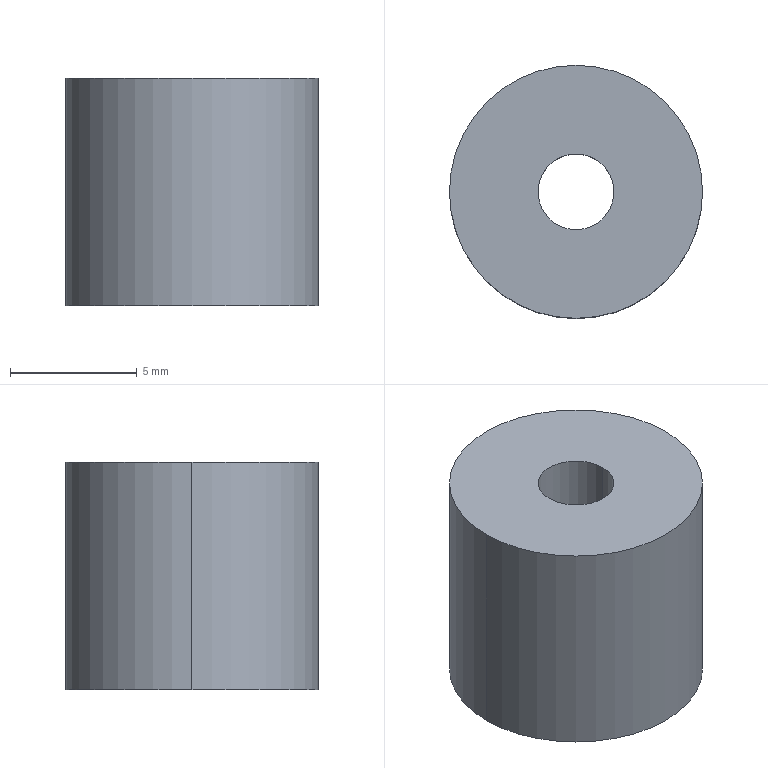Part | STEP file | 1 solid | 9 faces | box 10 x 10 x 9 mm | volume 537.212 mm3 | cylinder 6 | plane 3 | commonest cylinder face diameters 3 x2 6 x2 10 x2
STEP:
#1=CARTESIAN_POINT('',(0.,0.,0.));
#2=DIRECTION('',(0.,0.,1.));
#3=DIRECTION('',(1.,0.,0.));
#4=AXIS2_PLACEMENT_3D('',#1,#2,#3);
#5=CARTESIAN_POINT('',(1.5,0.,-4.));
#6=VERTEX_POINT('',#5);
#7=CARTESIAN_POINT('',(1.5,0.,0.));
#8=VERTEX_POINT('',#7);
#9=CARTESIAN_POINT('',(1.5,0.,0.));
#10=DIRECTION('',(0.,0.,1.));
#11=VECTOR('',#10,1.);
#12=LINE('',#9,#11);
#13=CARTESIAN_POINT('',(0.,0.,0.));
#14=DIRECTION('',(0.,0.,1.));
#15=DIRECTION('',(1.,0.,0.));
#16=AXIS2_PLACEMENT_3D('',#13,#14,#15);
#17=CYLINDRICAL_SURFACE('',#16,1.5);
#18=CARTESIAN_POINT('',(6.283,0.));
#19=DIRECTION('',(0.,1.));
#20=VECTOR('',#19,1.);
#21=LINE('',#18,#20);
#22=(GEOMETRIC_REPRESENTATION_CONTEXT(2)PARAMETRIC_REPRESENTATION_CONTEXT()REPRESENTATION_CONTEXT('',''));
#23=DEFINITIONAL_REPRESENTATION('',(#21),#22);
#24=PCURVE('',#17,#23);
#25=CARTESIAN_POINT('',(0.,0.,0.));
#26=DIRECTION('',(0.,0.,1.));
#27=DIRECTION('',(1.,0.,0.));
#28=AXIS2_PLACEMENT_3D('',#25,#26,#27);
#29=CYLINDRICAL_SURFACE('',#28,1.5);
#30=CARTESIAN_POINT('',(0.,0.));
#31=DIRECTION('',(0.,1.));
#32=VECTOR('',#31,1.);
#33=LINE('',#30,#32);
#34=(GEOMETRIC_REPRESENTATION_CONTEXT(2)PARAMETRIC_REPRESENTATION_CONTEXT()REPRESENTATION_CONTEXT('',''));
#35=DEFINITIONAL_REPRESENTATION('',(#33),#34);
#36=PCURVE('',#29,#35);
#37=SURFACE_CURVE('',#12,(#24,#36),.PCURVE_S1.);
#38=EDGE_CURVE('',#6,#8,#37,.T.);
#39=ORIENTED_EDGE('',*,*,#38,.T.);
#40=CARTESIAN_POINT('',(-1.5,0.,0.));
#41=VERTEX_POINT('',#40);
#42=CARTESIAN_POINT('',(0.,0.,0.));
#43=DIRECTION('',(0.,0.,1.));
#44=DIRECTION('',(1.,0.,0.));
#45=AXIS2_PLACEMENT_3D('',#42,#43,#44);
#46=CIRCLE('',#45,1.5);
#47=CARTESIAN_POINT('',(0.,0.));
#48=DIRECTION('',(1.,0.));
#49=VECTOR('',#48,1.);
#50=LINE('',#47,#49);
#51=(GEOMETRIC_REPRESENTATION_CONTEXT(2)PARAMETRIC_REPRESENTATION_CONTEXT()REPRESENTATION_CONTEXT('',''));
#52=DEFINITIONAL_REPRESENTATION('',(#50),#51);
#53=PCURVE('',#17,#52);
#54=CARTESIAN_POINT('',(1.5,0.,0.));
#55=DIRECTION('',(0.,0.,1.));
#56=DIRECTION('',(1.,0.,0.));
#57=AXIS2_PLACEMENT_3D('',#54,#55,#56);
#58=PLANE('',#57);
#59=CARTESIAN_POINT('',(-1.5,0.));
#60=DIRECTION('',(1.,0.));
#61=AXIS2_PLACEMENT_2D('',#59,#60);
#62=CIRCLE('',#61,1.5);
#63=(GEOMETRIC_REPRESENTATION_CONTEXT(2)PARAMETRIC_REPRESENTATION_CONTEXT()REPRESENTATION_CONTEXT('',''));
#64=DEFINITIONAL_REPRESENTATION('',(#62),#63);
#65=PCURVE('',#58,#64);
#66=SURFACE_CURVE('',#46,(#53,#65),.PCURVE_S1.);
#67=EDGE_CURVE('',#41,#8,#66,.T.);
#68=ORIENTED_EDGE('',*,*,#67,.F.);
#69=CARTESIAN_POINT('',(-1.5,0.,-4.));
#70=VERTEX_POINT('',#69);
#71=CARTESIAN_POINT('',(-1.5,0.,0.));
#72=DIRECTION('',(0.,0.,1.));
#73=VECTOR('',#72,1.);
#74=LINE('',#71,#73);
#75=CARTESIAN_POINT('',(3.142,0.));
#76=DIRECTION('',(0.,1.));
#77=VECTOR('',#76,1.);
#78=LINE('',#75,#77);
#79=(GEOMETRIC_REPRESENTATION_CONTEXT(2)PARAMETRIC_REPRESENTATION_CONTEXT()REPRESENTATION_CONTEXT('',''));
#80=DEFINITIONAL_REPRESENTATION('',(#78),#79);
#81=PCURVE('',#17,#80);
#82=CARTESIAN_POINT('',(3.142,0.));
#83=DIRECTION('',(0.,1.));
#84=VECTOR('',#83,1.);
#85=LINE('',#82,#84);
#86=(GEOMETRIC_REPRESENTATION_CONTEXT(2)PARAMETRIC_REPRESENTATION_CONTEXT()REPRESENTATION_CONTEXT('',''));
#87=DEFINITIONAL_REPRESENTATION('',(#85),#86);
#88=PCURVE('',#29,#87);
#89=SURFACE_CURVE('',#74,(#81,#88),.PCURVE_S1.);
#90=EDGE_CURVE('',#70,#41,#89,.T.);
#91=ORIENTED_EDGE('',*,*,#90,.F.);
#92=CARTESIAN_POINT('',(0.,0.,-4.));
#93=DIRECTION('',(0.,0.,1.));
#94=DIRECTION('',(1.,0.,0.));
#95=AXIS2_PLACEMENT_3D('',#92,#93,#94);
#96=CIRCLE('',#95,1.5);
#97=CARTESIAN_POINT('',(0.,-4.));
#98=DIRECTION('',(1.,0.));
#99=VECTOR('',#98,1.);
#100=LINE('',#97,#99);
#101=(GEOMETRIC_REPRESENTATION_CONTEXT(2)PARAMETRIC_REPRESENTATION_CONTEXT()REPRESENTATION_CONTEXT('',''));
#102=DEFINITIONAL_REPRESENTATION('',(#100),#101);
#103=PCURVE('',#17,#102);
#104=CARTESIAN_POINT('',(3.,0.,-4.));
#105=DIRECTION('',(0.,0.,-1.));
#106=DIRECTION('',(-1.,0.,0.));
#107=AXIS2_PLACEMENT_3D('',#104,#105,#106);
#108=PLANE('',#107);
#109=CARTESIAN_POINT('',(1.5,0.));
#110=CARTESIAN_POINT('',(1.5,2.598));
#111=CARTESIAN_POINT('',(3.75,1.299));
#112=CARTESIAN_POINT('',(6.,0.));
#113=CARTESIAN_POINT('',(3.75,-1.299));
#114=CARTESIAN_POINT('',(1.5,-2.598));
#115=CARTESIAN_POINT('',(1.5,0.));
#116=(BOUNDED_CURVE()B_SPLINE_CURVE(2,(#109,#110,#111,#112,#113,#114,#115),.UNSPECIFIED.,.T.,.F.)B_SPLINE_CURVE_WITH_KNOTS((1,2,2,2,2,1),(-2.094,0.,2.094,4.189,6.283,8.378),.UNSPECIFIED.)CURVE()GEOMETRIC_REPRESENTATION_ITEM()RATIONAL_B_SPLINE_CURVE((1.,0.5,1.,0.5,1.,0.5,1.))REPRESENTATION_ITEM(''));
#117=(GEOMETRIC_REPRESENTATION_CONTEXT(2)PARAMETRIC_REPRESENTATION_CONTEXT()REPRESENTATION_CONTEXT('',''));
#118=DEFINITIONAL_REPRESENTATION('',(#116),#117);
#119=PCURVE('',#108,#118);
#120=SURFACE_CURVE('',#96,(#103,#119),.PCURVE_S1.);
#121=EDGE_CURVE('',#70,#6,#120,.T.);
#122=ORIENTED_EDGE('',*,*,#121,.T.);
#123=EDGE_LOOP('',(#39,#68,#91,#122));
#124=FACE_BOUND('',#123,.F.);
#125=ADVANCED_FACE('',(#124),#17,.F.);
#126=CARTESIAN_POINT('',(3.,0.,-9.));
#127=VERTEX_POINT('',#126);
#128=CARTESIAN_POINT('',(3.,0.,-4.));
#129=VERTEX_POINT('',#128);
#130=CARTESIAN_POINT('',(3.,0.,0.));
#131=DIRECTION('',(0.,0.,1.));
#132=VECTOR('',#131,1.);
#133=LINE('',#130,#132);
#134=CARTESIAN_POINT('',(0.,0.,0.));
#135=DIRECTION('',(0.,0.,1.));
#136=DIRECTION('',(1.,0.,0.));
#137=AXIS2_PLACEMENT_3D('',#134,#135,#136);
#138=CYLINDRICAL_SURFACE('',#137,3.);
#139=CARTESIAN_POINT('',(6.283,0.));
#140=DIRECTION('',(0.,1.));
#141=VECTOR('',#140,1.);
#142=LINE('',#139,#141);
#143=(GEOMETRIC_REPRESENTATION_CONTEXT(2)PARAMETRIC_REPRESENTATION_CONTEXT()REPRESENTATION_CONTEXT('',''));
#144=DEFINITIONAL_REPRESENTATION('',(#142),#143);
#145=PCURVE('',#138,#144);
#146=CARTESIAN_POINT('',(0.,0.,0.));
#147=DIRECTION('',(0.,0.,1.));
#148=DIRECTION('',(1.,0.,0.));
#149=AXIS2_PLACEMENT_3D('',#146,#147,#148);
#150=CYLINDRICAL_SURFACE('',#149,3.);
#151=CARTESIAN_POINT('',(0.,0.));
#152=DIRECTION('',(0.,1.));
#153=VECTOR('',#152,1.);
#154=LINE('',#151,#153);
#155=(GEOMETRIC_REPRESENTATION_CONTEXT(2)PARAMETRIC_REPRESENTATION_CONTEXT()REPRESENTATION_CONTEXT('',''));
#156=DEFINITIONAL_REPRESENTATION('',(#154),#155);
#157=PCURVE('',#150,#156);
#158=SURFACE_CURVE('',#133,(#145,#157),.PCURVE_S1.);
#159=EDGE_CURVE('',#127,#129,#158,.T.);
#160=ORIENTED_EDGE('',*,*,#159,.T.);
#161=CARTESIAN_POINT('',(-3.,0.,-4.));
#162=VERTEX_POINT('',#161);
#163=CARTESIAN_POINT('',(0.,0.,-4.));
#164=DIRECTION('',(0.,0.,1.));
#165=DIRECTION('',(1.,0.,0.));
#166=AXIS2_PLACEMENT_3D('',#163,#164,#165);
#167=CIRCLE('',#166,3.);
#168=CARTESIAN_POINT('',(0.,-4.));
#169=DIRECTION('',(1.,0.));
#170=VECTOR('',#169,1.);
#171=LINE('',#168,#170);
#172=(GEOMETRIC_REPRESENTATION_CONTEXT(2)PARAMETRIC_REPRESENTATION_CONTEXT()REPRESENTATION_CONTEXT('',''));
#173=DEFINITIONAL_REPRESENTATION('',(#171),#172);
#174=PCURVE('',#138,#173);
#175=CARTESIAN_POINT('',(0.,0.));
#176=CARTESIAN_POINT('',(0.,5.196));
#177=CARTESIAN_POINT('',(4.5,2.598));
#178=CARTESIAN_POINT('',(9.,0.));
#179=CARTESIAN_POINT('',(4.5,-2.598));
#180=CARTESIAN_POINT('',(0.,-5.196));
#181=CARTESIAN_POINT('',(0.,0.));
#182=(BOUNDED_CURVE()B_SPLINE_CURVE(2,(#175,#176,#177,#178,#179,#180,#181),.UNSPECIFIED.,.T.,.F.)B_SPLINE_CURVE_WITH_KNOTS((1,2,2,2,2,1),(-2.094,0.,2.094,4.189,6.283,8.378),.UNSPECIFIED.)CURVE()GEOMETRIC_REPRESENTATION_ITEM()RATIONAL_B_SPLINE_CURVE((1.,0.5,1.,0.5,1.,0.5,1.))REPRESENTATION_ITEM(''));
#183=(GEOMETRIC_REPRESENTATION_CONTEXT(2)PARAMETRIC_REPRESENTATION_CONTEXT()REPRESENTATION_CONTEXT('',''));
#184=DEFINITIONAL_REPRESENTATION('',(#182),#183);
#185=PCURVE('',#108,#184);
#186=SURFACE_CURVE('',#167,(#174,#185),.PCURVE_S1.);
#187=EDGE_CURVE('',#162,#129,#186,.T.);
#188=ORIENTED_EDGE('',*,*,#187,.F.);
#189=CARTESIAN_POINT('',(-3.,0.,-9.));
#190=VERTEX_POINT('',#189);
#191=CARTESIAN_POINT('',(-3.,0.,0.));
#192=DIRECTION('',(0.,0.,1.));
#193=VECTOR('',#192,1.);
#194=LINE('',#191,#193);
#195=CARTESIAN_POINT('',(3.142,0.));
#196=DIRECTION('',(0.,1.));
#197=VECTOR('',#196,1.);
#198=LINE('',#195,#197);
#199=(GEOMETRIC_REPRESENTATION_CONTEXT(2)PARAMETRIC_REPRESENTATION_CONTEXT()REPRESENTATION_CONTEXT('',''));
#200=DEFINITIONAL_REPRESENTATION('',(#198),#199);
#201=PCURVE('',#138,#200);
#202=CARTESIAN_POINT('',(3.142,0.));
#203=DIRECTION('',(0.,1.));
#204=VECTOR('',#203,1.);
#205=LINE('',#202,#204);
#206=(GEOMETRIC_REPRESENTATION_CONTEXT(2)PARAMETRIC_REPRESENTATION_CONTEXT()REPRESENTATION_CONTEXT('',''));
#207=DEFINITIONAL_REPRESENTATION('',(#205),#206);
#208=PCURVE('',#150,#207);
#209=SURFACE_CURVE('',#194,(#201,#208),.PCURVE_S1.);
#210=EDGE_CURVE('',#190,#162,#209,.T.);
#211=ORIENTED_EDGE('',*,*,#210,.F.);
#212=CARTESIAN_POINT('',(0.,0.,-9.));
#213=DIRECTION('',(0.,0.,1.));
#214=DIRECTION('',(1.,0.,0.));
#215=AXIS2_PLACEMENT_3D('',#212,#213,#214);
#216=CIRCLE('',#215,3.);
#217=CARTESIAN_POINT('',(0.,-9.));
#218=DIRECTION('',(1.,0.));
#219=VECTOR('',#218,1.);
#220=LINE('',#217,#219);
#221=(GEOMETRIC_REPRESENTATION_CONTEXT(2)PARAMETRIC_REPRESENTATION_CONTEXT()REPRESENTATION_CONTEXT('',''));
#222=DEFINITIONAL_REPRESENTATION('',(#220),#221);
#223=PCURVE('',#138,#222);
#224=CARTESIAN_POINT('',(5.,0.,-9.));
#225=DIRECTION('',(0.,0.,-1.));
#226=DIRECTION('',(-1.,0.,0.));
#227=AXIS2_PLACEMENT_3D('',#224,#225,#226);
#228=PLANE('',#227);
#229=CARTESIAN_POINT('',(2.,0.));
#230=CARTESIAN_POINT('',(2.,5.196));
#231=CARTESIAN_POINT('',(6.5,2.598));
#232=CARTESIAN_POINT('',(11.,0.));
#233=CARTESIAN_POINT('',(6.5,-2.598));
#234=CARTESIAN_POINT('',(2.,-5.196));
#235=CARTESIAN_POINT('',(2.,0.));
#236=(BOUNDED_CURVE()B_SPLINE_CURVE(2,(#229,#230,#231,#232,#233,#234,#235),.UNSPECIFIED.,.T.,.F.)B_SPLINE_CURVE_WITH_KNOTS((1,2,2,2,2,1),(-2.094,0.,2.094,4.189,6.283,8.378),.UNSPECIFIED.)CURVE()GEOMETRIC_REPRESENTATION_ITEM()RATIONAL_B_SPLINE_CURVE((1.,0.5,1.,0.5,1.,0.5,1.))REPRESENTATION_ITEM(''));
#237=(GEOMETRIC_REPRESENTATION_CONTEXT(2)PARAMETRIC_REPRESENTATION_CONTEXT()REPRESENTATION_CONTEXT('',''));
#238=DEFINITIONAL_REPRESENTATION('',(#236),#237);
#239=PCURVE('',#228,#238);
#240=SURFACE_CURVE('',#216,(#223,#239),.PCURVE_S1.);
#241=EDGE_CURVE('',#190,#127,#240,.T.);
#242=ORIENTED_EDGE('',*,*,#241,.T.);
#243=EDGE_LOOP('',(#160,#188,#211,#242));
#244=FACE_BOUND('',#243,.F.);
#245=ADVANCED_FACE('',(#244),#138,.F.);
#246=CARTESIAN_POINT('',(5.,0.,-9.));
#247=VERTEX_POINT('',#246);
#248=CARTESIAN_POINT('',(-5.,0.,-9.));
#249=VERTEX_POINT('',#248);
#250=CARTESIAN_POINT('',(0.,0.,-9.));
#251=DIRECTION('',(0.,0.,1.));
#252=DIRECTION('',(1.,0.,0.));
#253=AXIS2_PLACEMENT_3D('',#250,#251,#252);
#254=CIRCLE('',#253,5.);
#255=CARTESIAN_POINT('',(0.,0.,0.));
#256=DIRECTION('',(0.,0.,1.));
#257=DIRECTION('',(1.,0.,0.));
#258=AXIS2_PLACEMENT_3D('',#255,#256,#257);
#259=CYLINDRICAL_SURFACE('',#258,5.);
#260=CARTESIAN_POINT('',(0.,-9.));
#261=DIRECTION('',(1.,0.));
#262=VECTOR('',#261,1.);
#263=LINE('',#260,#262);
#264=(GEOMETRIC_REPRESENTATION_CONTEXT(2)PARAMETRIC_REPRESENTATION_CONTEXT()REPRESENTATION_CONTEXT('',''));
#265=DEFINITIONAL_REPRESENTATION('',(#263),#264);
#266=PCURVE('',#259,#265);
#267=CARTESIAN_POINT('',(0.,0.));
#268=CARTESIAN_POINT('',(0.,8.66));
#269=CARTESIAN_POINT('',(7.5,4.33));
#270=CARTESIAN_POINT('',(15.,0.));
#271=CARTESIAN_POINT('',(7.5,-4.33));
#272=CARTESIAN_POINT('',(0.,-8.66));
#273=CARTESIAN_POINT('',(0.,0.));
#274=(BOUNDED_CURVE()B_SPLINE_CURVE(2,(#267,#268,#269,#270,#271,#272,#273),.UNSPECIFIED.,.T.,.F.)B_SPLINE_CURVE_WITH_KNOTS((1,2,2,2,2,1),(-2.094,0.,2.094,4.189,6.283,8.378),.UNSPECIFIED.)CURVE()GEOMETRIC_REPRESENTATION_ITEM()RATIONAL_B_SPLINE_CURVE((1.,0.5,1.,0.5,1.,0.5,1.))REPRESENTATION_ITEM(''));
#275=(GEOMETRIC_REPRESENTATION_CONTEXT(2)PARAMETRIC_REPRESENTATION_CONTEXT()REPRESENTATION_CONTEXT('',''));
#276=DEFINITIONAL_REPRESENTATION('',(#274),#275);
#277=PCURVE('',#228,#276);
#278=SURFACE_CURVE('',#254,(#266,#277),.PCURVE_S1.);
#279=EDGE_CURVE('',#247,#249,#278,.T.);
#280=ORIENTED_EDGE('',*,*,#279,.T.);
#281=CARTESIAN_POINT('',(-5.,0.,0.));
#282=VERTEX_POINT('',#281);
#283=CARTESIAN_POINT('',(-5.,0.,0.));
#284=DIRECTION('',(0.,0.,1.));
#285=VECTOR('',#284,1.);
#286=LINE('',#283,#285);
#287=CARTESIAN_POINT('',(3.142,0.));
#288=DIRECTION('',(0.,1.));
#289=VECTOR('',#288,1.);
#290=LINE('',#287,#289);
#291=(GEOMETRIC_REPRESENTATION_CONTEXT(2)PARAMETRIC_REPRESENTATION_CONTEXT()REPRESENTATION_CONTEXT('',''));
#292=DEFINITIONAL_REPRESENTATION('',(#290),#291);
#293=PCURVE('',#259,#292);
#294=CARTESIAN_POINT('',(0.,0.,0.));
#295=DIRECTION('',(0.,0.,1.));
#296=DIRECTION('',(1.,0.,0.));
#297=AXIS2_PLACEMENT_3D('',#294,#295,#296);
#298=CYLINDRICAL_SURFACE('',#297,5.);
#299=CARTESIAN_POINT('',(3.142,0.));
#300=DIRECTION('',(0.,1.));
#301=VECTOR('',#300,1.);
#302=LINE('',#299,#301);
#303=(GEOMETRIC_REPRESENTATION_CONTEXT(2)PARAMETRIC_REPRESENTATION_CONTEXT()REPRESENTATION_CONTEXT('',''));
#304=DEFINITIONAL_REPRESENTATION('',(#302),#303);
#305=PCURVE('',#298,#304);
#306=SURFACE_CURVE('',#286,(#293,#305),.PCURVE_S1.);
#307=EDGE_CURVE('',#249,#282,#306,.T.);
#308=ORIENTED_EDGE('',*,*,#307,.T.);
#309=CARTESIAN_POINT('',(5.,0.,0.));
#310=VERTEX_POINT('',#309);
#311=CARTESIAN_POINT('',(0.,0.,0.));
#312=DIRECTION('',(0.,0.,1.));
#313=DIRECTION('',(1.,0.,0.));
#314=AXIS2_PLACEMENT_3D('',#311,#312,#313);
#315=CIRCLE('',#314,5.);
#316=CARTESIAN_POINT('',(0.,0.));
#317=DIRECTION('',(1.,0.));
#318=VECTOR('',#317,1.);
#319=LINE('',#316,#318);
#320=(GEOMETRIC_REPRESENTATION_CONTEXT(2)PARAMETRIC_REPRESENTATION_CONTEXT()REPRESENTATION_CONTEXT('',''));
#321=DEFINITIONAL_REPRESENTATION('',(#319),#320);
#322=PCURVE('',#259,#321);
#323=CARTESIAN_POINT('',(-1.5,0.));
#324=DIRECTION('',(1.,0.));
#325=AXIS2_PLACEMENT_2D('',#323,#324);
#326=CIRCLE('',#325,5.);
#327=(GEOMETRIC_REPRESENTATION_CONTEXT(2)PARAMETRIC_REPRESENTATION_CONTEXT()REPRESENTATION_CONTEXT('',''));
#328=DEFINITIONAL_REPRESENTATION('',(#326),#327);
#329=PCURVE('',#58,#328);
#330=SURFACE_CURVE('',#315,(#322,#329),.PCURVE_S1.);
#331=EDGE_CURVE('',#310,#282,#330,.T.);
#332=ORIENTED_EDGE('',*,*,#331,.F.);
#333=CARTESIAN_POINT('',(5.,0.,0.));
#334=DIRECTION('',(0.,0.,1.));
#335=VECTOR('',#334,1.);
#336=LINE('',#333,#335);
#337=CARTESIAN_POINT('',(0.,0.));
#338=DIRECTION('',(0.,1.));
#339=VECTOR('',#338,1.);
#340=LINE('',#337,#339);
#341=(GEOMETRIC_REPRESENTATION_CONTEXT(2)PARAMETRIC_REPRESENTATION_CONTEXT()REPRESENTATION_CONTEXT('',''));
#342=DEFINITIONAL_REPRESENTATION('',(#340),#341);
#343=PCURVE('',#259,#342);
#344=CARTESIAN_POINT('',(6.283,0.));
#345=DIRECTION('',(0.,1.));
#346=VECTOR('',#345,1.);
#347=LINE('',#344,#346);
#348=(GEOMETRIC_REPRESENTATION_CONTEXT(2)PARAMETRIC_REPRESENTATION_CONTEXT()REPRESENTATION_CONTEXT('',''));
#349=DEFINITIONAL_REPRESENTATION('',(#347),#348);
#350=PCURVE('',#298,#349);
#351=SURFACE_CURVE('',#336,(#343,#350),.PCURVE_S1.);
#352=EDGE_CURVE('',#247,#310,#351,.T.);
#353=ORIENTED_EDGE('',*,*,#352,.F.);
#354=EDGE_LOOP('',(#280,#308,#332,#353));
#355=FACE_BOUND('',#354,.T.);
#356=ADVANCED_FACE('',(#355),#259,.T.);
#357=ORIENTED_EDGE('',*,*,#307,.F.);
#358=CARTESIAN_POINT('',(0.,0.,-9.));
#359=DIRECTION('',(0.,0.,1.));
#360=DIRECTION('',(1.,0.,0.));
#361=AXIS2_PLACEMENT_3D('',#358,#359,#360);
#362=CIRCLE('',#361,5.);
#363=CARTESIAN_POINT('',(0.,-9.));
#364=DIRECTION('',(1.,0.));
#365=VECTOR('',#364,1.);
#366=LINE('',#363,#365);
#367=(GEOMETRIC_REPRESENTATION_CONTEXT(2)PARAMETRIC_REPRESENTATION_CONTEXT()REPRESENTATION_CONTEXT('',''));
#368=DEFINITIONAL_REPRESENTATION('',(#366),#367);
#369=PCURVE('',#298,#368);
#370=CARTESIAN_POINT('',(0.,0.));
#371=CARTESIAN_POINT('',(0.,8.66));
#372=CARTESIAN_POINT('',(7.5,4.33));
#373=CARTESIAN_POINT('',(15.,0.));
#374=CARTESIAN_POINT('',(7.5,-4.33));
#375=CARTESIAN_POINT('',(0.,-8.66));
#376=CARTESIAN_POINT('',(0.,0.));
#377=(BOUNDED_CURVE()B_SPLINE_CURVE(2,(#370,#371,#372,#373,#374,#375,#376),.UNSPECIFIED.,.T.,.F.)B_SPLINE_CURVE_WITH_KNOTS((1,2,2,2,2,1),(-2.094,0.,2.094,4.189,6.283,8.378),.UNSPECIFIED.)CURVE()GEOMETRIC_REPRESENTATION_ITEM()RATIONAL_B_SPLINE_CURVE((1.,0.5,1.,0.5,1.,0.5,1.))REPRESENTATION_ITEM(''));
#378=(GEOMETRIC_REPRESENTATION_CONTEXT(2)PARAMETRIC_REPRESENTATION_CONTEXT()REPRESENTATION_CONTEXT('',''));
#379=DEFINITIONAL_REPRESENTATION('',(#377),#378);
#380=PCURVE('',#228,#379);
#381=SURFACE_CURVE('',#362,(#369,#380),.PCURVE_S1.);
#382=EDGE_CURVE('',#249,#247,#381,.T.);
#383=ORIENTED_EDGE('',*,*,#382,.T.);
#384=ORIENTED_EDGE('',*,*,#352,.T.);
#385=CARTESIAN_POINT('',(0.,0.,0.));
#386=DIRECTION('',(0.,0.,1.));
#387=DIRECTION('',(1.,0.,0.));
#388=AXIS2_PLACEMENT_3D('',#385,#386,#387);
#389=CIRCLE('',#388,5.);
#390=CARTESIAN_POINT('',(0.,0.));
#391=DIRECTION('',(1.,0.));
#392=VECTOR('',#391,1.);
#393=LINE('',#390,#392);
#394=(GEOMETRIC_REPRESENTATION_CONTEXT(2)PARAMETRIC_REPRESENTATION_CONTEXT()REPRESENTATION_CONTEXT('',''));
#395=DEFINITIONAL_REPRESENTATION('',(#393),#394);
#396=PCURVE('',#298,#395);
#397=CARTESIAN_POINT('',(-1.5,0.));
#398=DIRECTION('',(1.,0.));
#399=AXIS2_PLACEMENT_2D('',#397,#398);
#400=CIRCLE('',#399,5.);
#401=(GEOMETRIC_REPRESENTATION_CONTEXT(2)PARAMETRIC_REPRESENTATION_CONTEXT()REPRESENTATION_CONTEXT('',''));
#402=DEFINITIONAL_REPRESENTATION('',(#400),#401);
#403=PCURVE('',#58,#402);
#404=SURFACE_CURVE('',#389,(#396,#403),.PCURVE_S1.);
#405=EDGE_CURVE('',#282,#310,#404,.T.);
#406=ORIENTED_EDGE('',*,*,#405,.F.);
#407=EDGE_LOOP('',(#357,#383,#384,#406));
#408=FACE_BOUND('',#407,.T.);
#409=ADVANCED_FACE('',(#408),#298,.T.);
#410=CARTESIAN_POINT('',(0.,0.,-9.));
#411=DIRECTION('',(0.,0.,1.));
#412=DIRECTION('',(1.,0.,0.));
#413=AXIS2_PLACEMENT_3D('',#410,#411,#412);
#414=CIRCLE('',#413,3.);
#415=CARTESIAN_POINT('',(2.,0.));
#416=CARTESIAN_POINT('',(2.,5.196));
#417=CARTESIAN_POINT('',(6.5,2.598));
#418=CARTESIAN_POINT('',(11.,0.));
#419=CARTESIAN_POINT('',(6.5,-2.598));
#420=CARTESIAN_POINT('',(2.,-5.196));
#421=CARTESIAN_POINT('',(2.,0.));
#422=(BOUNDED_CURVE()B_SPLINE_CURVE(2,(#415,#416,#417,#418,#419,#420,#421),.UNSPECIFIED.,.T.,.F.)B_SPLINE_CURVE_WITH_KNOTS((1,2,2,2,2,1),(-2.094,0.,2.094,4.189,6.283,8.378),.UNSPECIFIED.)CURVE()GEOMETRIC_REPRESENTATION_ITEM()RATIONAL_B_SPLINE_CURVE((1.,0.5,1.,0.5,1.,0.5,1.))REPRESENTATION_ITEM(''));
#423=(GEOMETRIC_REPRESENTATION_CONTEXT(2)PARAMETRIC_REPRESENTATION_CONTEXT()REPRESENTATION_CONTEXT('',''));
#424=DEFINITIONAL_REPRESENTATION('',(#422),#423);
#425=PCURVE('',#228,#424);
#426=CARTESIAN_POINT('',(0.,-9.));
#427=DIRECTION('',(1.,0.));
#428=VECTOR('',#427,1.);
#429=LINE('',#426,#428);
#430=(GEOMETRIC_REPRESENTATION_CONTEXT(2)PARAMETRIC_REPRESENTATION_CONTEXT()REPRESENTATION_CONTEXT('',''));
#431=DEFINITIONAL_REPRESENTATION('',(#429),#430);
#432=PCURVE('',#150,#431);
#433=SURFACE_CURVE('',#414,(#425,#432),.PCURVE_S1.);
#434=EDGE_CURVE('',#127,#190,#433,.T.);
#435=ORIENTED_EDGE('',*,*,#434,.T.);
#436=ORIENTED_EDGE('',*,*,#241,.T.);
#437=EDGE_LOOP('',(#435,#436));
#438=FACE_BOUND('',#437,.T.);
#439=ORIENTED_EDGE('',*,*,#279,.F.);
#440=ORIENTED_EDGE('',*,*,#382,.F.);
#441=EDGE_LOOP('',(#439,#440));
#442=FACE_BOUND('',#441,.T.);
#443=ADVANCED_FACE('',(#438,#442),#228,.T.);
#444=CARTESIAN_POINT('',(0.,0.,-4.));
#445=DIRECTION('',(0.,0.,1.));
#446=DIRECTION('',(1.,0.,0.));
#447=AXIS2_PLACEMENT_3D('',#444,#445,#446);
#448=CIRCLE('',#447,3.);
#449=CARTESIAN_POINT('',(0.,-4.));
#450=DIRECTION('',(1.,0.));
#451=VECTOR('',#450,1.);
#452=LINE('',#449,#451);
#453=(GEOMETRIC_REPRESENTATION_CONTEXT(2)PARAMETRIC_REPRESENTATION_CONTEXT()REPRESENTATION_CONTEXT('',''));
#454=DEFINITIONAL_REPRESENTATION('',(#452),#453);
#455=PCURVE('',#150,#454);
#456=CARTESIAN_POINT('',(0.,0.));
#457=CARTESIAN_POINT('',(0.,5.196));
#458=CARTESIAN_POINT('',(4.5,2.598));
#459=CARTESIAN_POINT('',(9.,0.));
#460=CARTESIAN_POINT('',(4.5,-2.598));
#461=CARTESIAN_POINT('',(0.,-5.196));
#462=CARTESIAN_POINT('',(0.,0.));
#463=(BOUNDED_CURVE()B_SPLINE_CURVE(2,(#456,#457,#458,#459,#460,#461,#462),.UNSPECIFIED.,.T.,.F.)B_SPLINE_CURVE_WITH_KNOTS((1,2,2,2,2,1),(-2.094,0.,2.094,4.189,6.283,8.378),.UNSPECIFIED.)CURVE()GEOMETRIC_REPRESENTATION_ITEM()RATIONAL_B_SPLINE_CURVE((1.,0.5,1.,0.5,1.,0.5,1.))REPRESENTATION_ITEM(''));
#464=(GEOMETRIC_REPRESENTATION_CONTEXT(2)PARAMETRIC_REPRESENTATION_CONTEXT()REPRESENTATION_CONTEXT('',''));
#465=DEFINITIONAL_REPRESENTATION('',(#463),#464);
#466=PCURVE('',#108,#465);
#467=SURFACE_CURVE('',#448,(#455,#466),.PCURVE_S1.);
#468=EDGE_CURVE('',#129,#162,#467,.T.);
#469=ORIENTED_EDGE('',*,*,#468,.F.);
#470=ORIENTED_EDGE('',*,*,#159,.F.);
#471=ORIENTED_EDGE('',*,*,#434,.T.);
#472=ORIENTED_EDGE('',*,*,#210,.T.);
#473=EDGE_LOOP('',(#469,#470,#471,#472));
#474=FACE_BOUND('',#473,.F.);
#475=ADVANCED_FACE('',(#474),#150,.F.);
#476=CARTESIAN_POINT('',(0.,0.,-4.));
#477=DIRECTION('',(0.,0.,1.));
#478=DIRECTION('',(1.,0.,0.));
#479=AXIS2_PLACEMENT_3D('',#476,#477,#478);
#480=CIRCLE('',#479,1.5);
#481=CARTESIAN_POINT('',(1.5,0.));
#482=CARTESIAN_POINT('',(1.5,2.598));
#483=CARTESIAN_POINT('',(3.75,1.299));
#484=CARTESIAN_POINT('',(6.,0.));
#485=CARTESIAN_POINT('',(3.75,-1.299));
#486=CARTESIAN_POINT('',(1.5,-2.598));
#487=CARTESIAN_POINT('',(1.5,0.));
#488=(BOUNDED_CURVE()B_SPLINE_CURVE(2,(#481,#482,#483,#484,#485,#486,#487),.UNSPECIFIED.,.T.,.F.)B_SPLINE_CURVE_WITH_KNOTS((1,2,2,2,2,1),(-2.094,0.,2.094,4.189,6.283,8.378),.UNSPECIFIED.)CURVE()GEOMETRIC_REPRESENTATION_ITEM()RATIONAL_B_SPLINE_CURVE((1.,0.5,1.,0.5,1.,0.5,1.))REPRESENTATION_ITEM(''));
#489=(GEOMETRIC_REPRESENTATION_CONTEXT(2)PARAMETRIC_REPRESENTATION_CONTEXT()REPRESENTATION_CONTEXT('',''));
#490=DEFINITIONAL_REPRESENTATION('',(#488),#489);
#491=PCURVE('',#108,#490);
#492=CARTESIAN_POINT('',(0.,-4.));
#493=DIRECTION('',(1.,0.));
#494=VECTOR('',#493,1.);
#495=LINE('',#492,#494);
#496=(GEOMETRIC_REPRESENTATION_CONTEXT(2)PARAMETRIC_REPRESENTATION_CONTEXT()REPRESENTATION_CONTEXT('',''));
#497=DEFINITIONAL_REPRESENTATION('',(#495),#496);
#498=PCURVE('',#29,#497);
#499=SURFACE_CURVE('',#480,(#491,#498),.PCURVE_S1.);
#500=EDGE_CURVE('',#6,#70,#499,.T.);
#501=ORIENTED_EDGE('',*,*,#500,.T.);
#502=ORIENTED_EDGE('',*,*,#121,.T.);
#503=EDGE_LOOP('',(#501,#502));
#504=FACE_BOUND('',#503,.T.);
#505=ORIENTED_EDGE('',*,*,#468,.F.);
#506=ORIENTED_EDGE('',*,*,#187,.F.);
#507=EDGE_LOOP('',(#505,#506));
#508=FACE_BOUND('',#507,.T.);
#509=ADVANCED_FACE('',(#504,#508),#108,.T.);
#510=CARTESIAN_POINT('',(0.,0.,0.));
#511=DIRECTION('',(0.,0.,1.));
#512=DIRECTION('',(1.,0.,0.));
#513=AXIS2_PLACEMENT_3D('',#510,#511,#512);
#514=CIRCLE('',#513,1.5);
#515=CARTESIAN_POINT('',(0.,0.));
#516=DIRECTION('',(1.,0.));
#517=VECTOR('',#516,1.);
#518=LINE('',#515,#517);
#519=(GEOMETRIC_REPRESENTATION_CONTEXT(2)PARAMETRIC_REPRESENTATION_CONTEXT()REPRESENTATION_CONTEXT('',''));
#520=DEFINITIONAL_REPRESENTATION('',(#518),#519);
#521=PCURVE('',#29,#520);
#522=CARTESIAN_POINT('',(-1.5,0.));
#523=DIRECTION('',(1.,0.));
#524=AXIS2_PLACEMENT_2D('',#522,#523);
#525=CIRCLE('',#524,1.5);
#526=(GEOMETRIC_REPRESENTATION_CONTEXT(2)PARAMETRIC_REPRESENTATION_CONTEXT()REPRESENTATION_CONTEXT('',''));
#527=DEFINITIONAL_REPRESENTATION('',(#525),#526);
#528=PCURVE('',#58,#527);
#529=SURFACE_CURVE('',#514,(#521,#528),.PCURVE_S1.);
#530=EDGE_CURVE('',#8,#41,#529,.T.);
#531=ORIENTED_EDGE('',*,*,#530,.F.);
#532=ORIENTED_EDGE('',*,*,#38,.F.);
#533=ORIENTED_EDGE('',*,*,#500,.T.);
#534=ORIENTED_EDGE('',*,*,#90,.T.);
#535=EDGE_LOOP('',(#531,#532,#533,#534));
#536=FACE_BOUND('',#535,.F.);
#537=ADVANCED_FACE('',(#536),#29,.F.);
#538=ORIENTED_EDGE('',*,*,#331,.T.);
#539=ORIENTED_EDGE('',*,*,#405,.T.);
#540=EDGE_LOOP('',(#538,#539));
#541=FACE_BOUND('',#540,.T.);
#542=ORIENTED_EDGE('',*,*,#530,.F.);
#543=ORIENTED_EDGE('',*,*,#67,.F.);
#544=EDGE_LOOP('',(#542,#543));
#545=FACE_BOUND('',#544,.T.);
#546=ADVANCED_FACE('',(#541,#545),#58,.T.);
#547=CLOSED_SHELL('',(#125,#245,#356,#409,#443,#475,#509,#537,#546));
#548=MANIFOLD_SOLID_BREP('',#547);
#549=(LENGTH_UNIT()NAMED_UNIT(*)SI_UNIT(.MILLI.,.METRE.));
#550=UNCERTAINTY_MEASURE_WITH_UNIT(LENGTH_MEASURE(0.0000001),#549,'','');
#551=(NAMED_UNIT(*)PLANE_ANGLE_UNIT()SI_UNIT($,.RADIAN.));
#552=(NAMED_UNIT(*)SI_UNIT($,.STERADIAN.)SOLID_ANGLE_UNIT());
#553=(GEOMETRIC_REPRESENTATION_CONTEXT(3)GLOBAL_UNCERTAINTY_ASSIGNED_CONTEXT((#550))GLOBAL_UNIT_ASSIGNED_CONTEXT((#549,#551,#552))REPRESENTATION_CONTEXT('',''));
#554=ADVANCED_BREP_SHAPE_REPRESENTATION('',(#4,#548),#553);